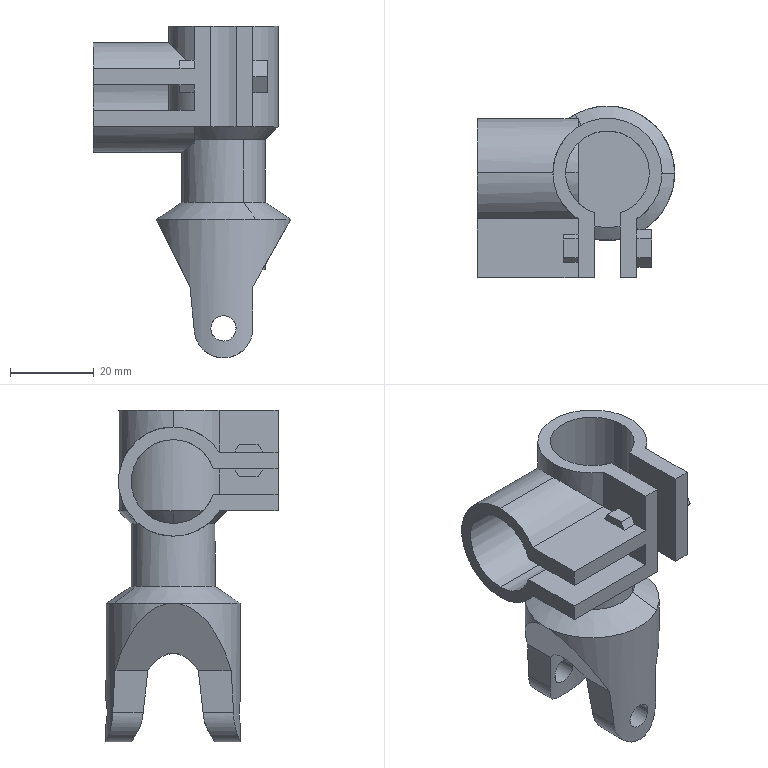Part | SolidWorks | features MBimport 1 | 1 solid | 80 faces | box 47 x 41 x 79 mm | volume 34473 mm3 | plane 41 | cylinder 32 | cone 7 | commonest cylinder face diameters 20 x15 26 x9 6 x4 14 x2 32 x2